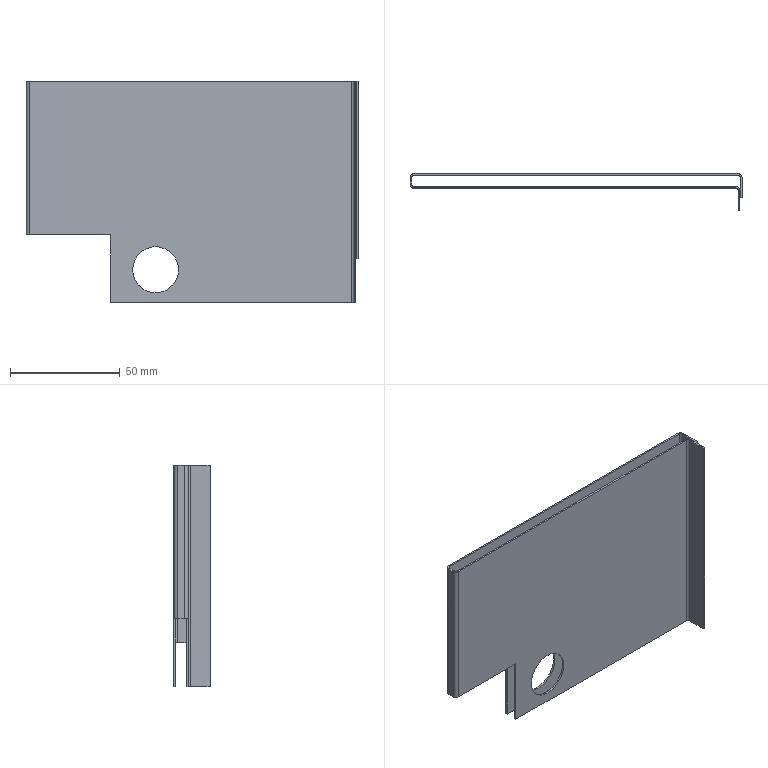Part | STEP file | 64563181 | 1 solid | 50 faces | box 151.5 x 16.5 x 101 mm | volume 21611 mm3 | plane 36 | cylinder 14 | commonest cylinder face diameters 2 x4 3.5 x4 21 x4 4 x2